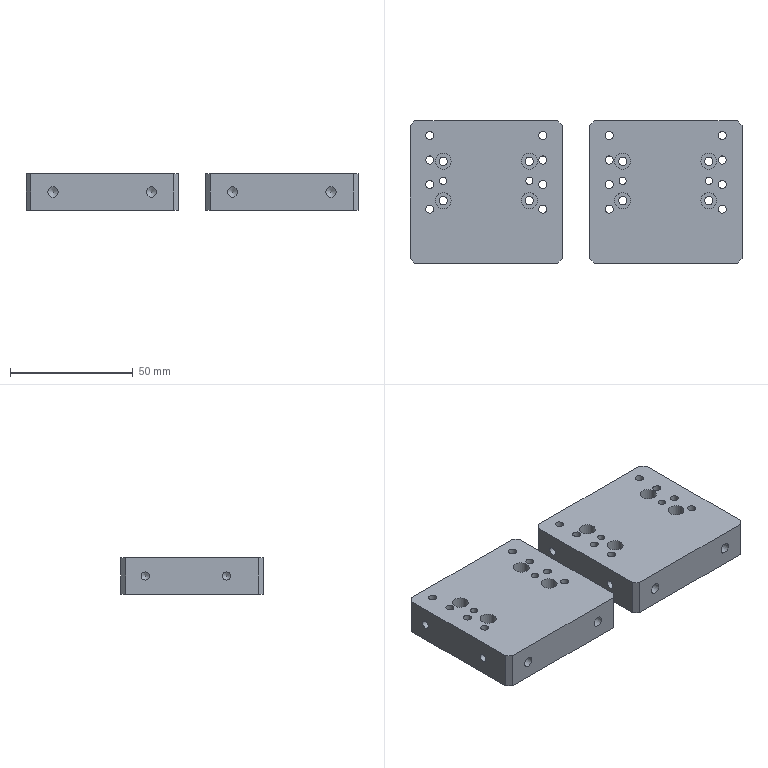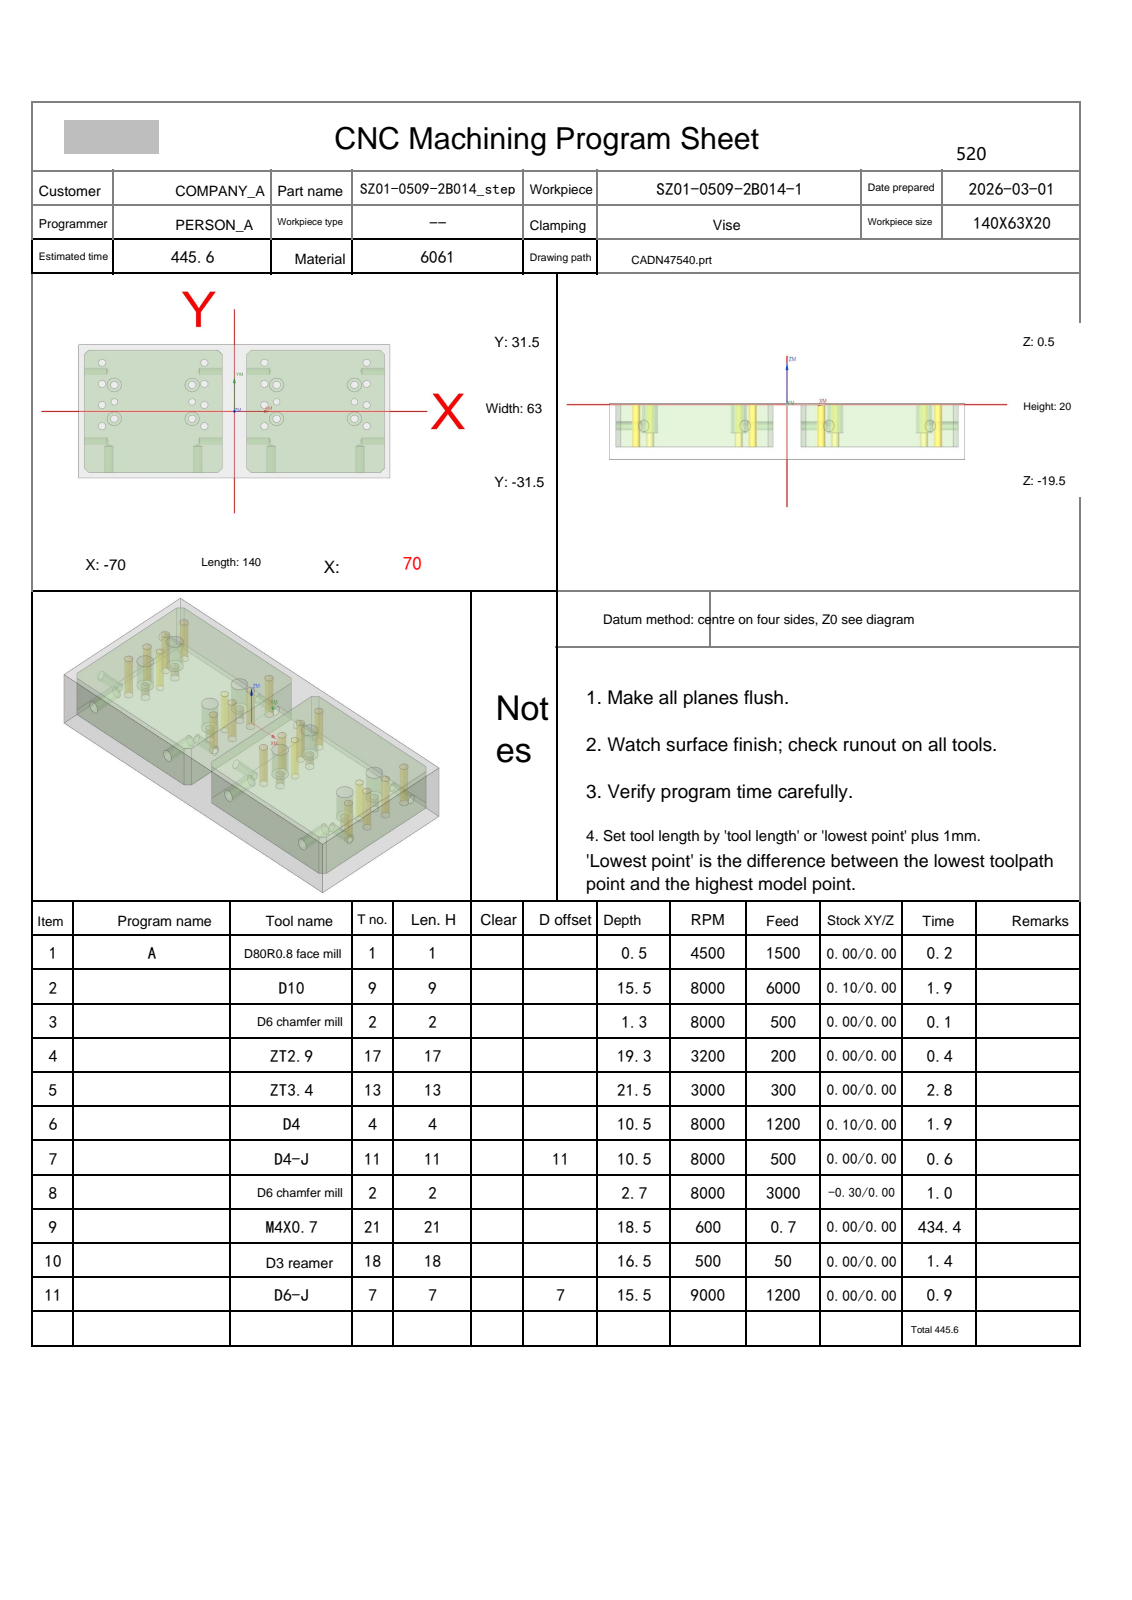NC program | NX | posted by the shop | part box 135 x 58 x 15 mm
Lines 1 to 1865 of 1983, first 1190 of 1863 lines:
%
O0001
(Machine time: 858.92 MIN)
(===Total Tool:10===)
(T1=D80R0.8 face mill D=80.  R=0.8  D-  H01 Z=0.    )
(T9=D10     D=10.  R=0.   D-  H09 Z=-15.  )
(T2=D6 chamfer mill   D=6.   R=0.   D-  H02 Z=-2.2  )
(T17=ZT2.9  D=2.9  DR_a=120 D-  H17 Z=-18.84)
(T13=ZT3.4  D=3.4  DR_a=118 D-  H13 Z=-21.  )
(T4=D4      D=4.   R=0.   D-  H04 Z=-10.  )
(T11=D4-J   D=4.   R=0.   D11 H11 Z=-10.  )
(T21=M4X0.7 D=3.3  DR_a=180 D-  H21 Z=-18.  )
(T18=D3 reamer   D=3.   DR_a=180 D-  H18 Z=-16.  )
(T7=D6-J    D=6.   R=0.   D7  H07 Z=-15.  )
G80 G90 G17 G49 G40
G91 G28 Z0
M01
N1 T01 M06
(D80R0.8 face mill  D=80. R=0.8 H=01 ce=0.00 di=0.00)
G00 G90 G54 X-112.5 Y0.0 M03 S4500
G43 H01 Z50.
M08
Z2.
G01 Z0.0 F1500.
X-107.5
X107.5
X112.5
Z2.
G00 Z50.
G91 G28 Z0.0
M05
M09
G91 G28 Z0.0
M01
N2 T09 M06
(D10  D=10. R=0. H=09 ce=0.10 di=0.00)
G00 G90 G54 X36.5 Y34.1 M03 S8000
G43 H09 Z50.
M08
Z.5
G01 X65.5 Z.416 F6000.
G02 X69.106 Y32.606 Z.404 I0.0 J-5.1
G01 X71.106 Y30.606 Z.396
G02 X72.6 Y27. Z.385 I-3.606 J-3.606
G01 Y-27. Z.228
G02 X71.106 Y-30.606 Z.216 I-5.1 J0.0
G01 X69.106 Y-32.606 Z.208
G02 X65.5 Y-34.1 Z.197 I-3.606 J3.606
G01 X7.5 Z.028
G02 X3.894 Y-32.606 Z.017 I0.0 J5.1
G01 X1.894 Y-30.606 Z.009
G02 X.4 Y-27. Z-.003 I3.606 J3.606
G01 Y27. Z-.16
G02 X1.894 Y30.606 Z-.171 I5.1 J0.0
G01 X3.894 Y32.606 Z-.179
G02 X7.5 Y34.1 Z-.191 I3.606 J-3.606
G01 X65.5 Z-.359
G02 X69.106 Y32.606 Z-.371 I0.0 J-5.1
G01 X71.106 Y30.606 Z-.379
G02 X72.6 Y27. Z-.39 I-3.606 J-3.606
G01 Y-27. Z-.547
G02 X71.106 Y-30.606 Z-.559 I-5.1 J0.0
G01 X69.106 Y-32.606 Z-.567
G02 X65.5 Y-34.1 Z-.578 I-3.606 J3.606
G01 X7.5 Z-.747
G02 X3.894 Y-32.606 Z-.758 I0.0 J5.1
G01 X1.894 Y-30.606 Z-.766
G02 X.4 Y-27. Z-.778 I3.606 J3.606
G01 Y27. Z-.935
G02 X1.894 Y30.606 Z-.946 I5.1 J0.0
G01 X3.894 Y32.606 Z-.954
G02 X7.5 Y34.1 Z-.966 I3.606 J-3.606
G01 X65.5 Z-1.134
G02 X69.106 Y32.606 Z-1.146 I0.0 J-5.1
G01 X71.106 Y30.606 Z-1.154
G02 X72.6 Y27. Z-1.165 I-3.606 J-3.606
G01 Y-27. Z-1.322
G02 X71.106 Y-30.606 Z-1.334 I-5.1 J0.0
G01 X69.106 Y-32.606 Z-1.342
G02 X65.5 Y-34.1 Z-1.353 I-3.606 J3.606
G01 X7.5 Z-1.522
G02 X3.894 Y-32.606 Z-1.533 I0.0 J5.1
G01 X1.894 Y-30.606 Z-1.541
G02 X.4 Y-27. Z-1.553 I3.606 J3.606
G01 Y27. Z-1.71
G02 X1.894 Y30.606 Z-1.721 I5.1 J0.0
G01 X3.894 Y32.606 Z-1.729
G02 X7.5 Y34.1 Z-1.741 I3.606 J-3.606
G01 X65.5 Z-1.909
G02 X69.106 Y32.606 Z-1.921 I0.0 J-5.1
G01 X71.106 Y30.606 Z-1.929
G02 X72.6 Y27. Z-1.94 I-3.606 J-3.606
G01 Y-27. Z-2.097
G02 X71.106 Y-30.606 Z-2.109 I-5.1 J0.0
G01 X69.106 Y-32.606 Z-2.117
G02 X65.5 Y-34.1 Z-2.128 I-3.606 J3.606
G01 X7.5 Z-2.297
G02 X3.894 Y-32.606 Z-2.308 I0.0 J5.1
G01 X1.894 Y-30.606 Z-2.316
G02 X.4 Y-27. Z-2.328 I3.606 J3.606
G01 Y27. Z-2.485
G02 X1.894 Y30.606 Z-2.496 I5.1 J0.0
G01 X3.894 Y32.606 Z-2.504
G02 X7.5 Y34.1 Z-2.516 I3.606 J-3.606
G01 X65.5 Z-2.684
G02 X69.106 Y32.606 Z-2.696 I0.0 J-5.1
G01 X71.106 Y30.606 Z-2.704
G02 X72.6 Y27. Z-2.715 I-3.606 J-3.606
G01 Y-27. Z-2.872
G02 X71.106 Y-30.606 Z-2.884 I-5.1 J0.0
G01 X69.106 Y-32.606 Z-2.892
G02 X65.5 Y-34.1 Z-2.903 I-3.606 J3.606
G01 X7.5 Z-3.072
G02 X3.894 Y-32.606 Z-3.083 I0.0 J5.1
G01 X1.894 Y-30.606 Z-3.091
G02 X.4 Y-27. Z-3.103 I3.606 J3.606
G01 Y27. Z-3.26
G02 X1.894 Y30.606 Z-3.271 I5.1 J0.0
G01 X3.894 Y32.606 Z-3.279
G02 X7.5 Y34.1 Z-3.291 I3.606 J-3.606
G01 X65.5 Z-3.459
G02 X69.106 Y32.606 Z-3.471 I0.0 J-5.1
G01 X71.106 Y30.606 Z-3.479
G02 X72.6 Y27. Z-3.49 I-3.606 J-3.606
G01 Y-27. Z-3.647
G02 X71.106 Y-30.606 Z-3.659 I-5.1 J0.0
G01 X69.106 Y-32.606 Z-3.667
G02 X65.5 Y-34.1 Z-3.678 I-3.606 J3.606
G01 X7.5 Z-3.847
G02 X3.894 Y-32.606 Z-3.858 I0.0 J5.1
G01 X1.894 Y-30.606 Z-3.866
G02 X.4 Y-27. Z-3.878 I3.606 J3.606
G01 Y27. Z-4.035
G02 X1.894 Y30.606 Z-4.046 I5.1 J0.0
G01 X3.894 Y32.606 Z-4.054
G02 X7.5 Y34.1 Z-4.066 I3.606 J-3.606
G01 X65.5 Z-4.234
G02 X69.106 Y32.606 Z-4.246 I0.0 J-5.1
G01 X71.106 Y30.606 Z-4.254
G02 X72.6 Y27. Z-4.265 I-3.606 J-3.606
G01 Y-27. Z-4.422
G02 X71.106 Y-30.606 Z-4.434 I-5.1 J0.0
G01 X69.106 Y-32.606 Z-4.442
G02 X65.5 Y-34.1 Z-4.453 I-3.606 J3.606
G01 X7.5 Z-4.622
G02 X3.894 Y-32.606 Z-4.633 I0.0 J5.1
G01 X1.894 Y-30.606 Z-4.641
G02 X.4 Y-27. Z-4.653 I3.606 J3.606
G01 Y27. Z-4.81
G02 X1.894 Y30.606 Z-4.821 I5.1 J0.0
G01 X3.894 Y32.606 Z-4.829
G02 X7.5 Y34.1 Z-4.841 I3.606 J-3.606
G01 X65.5 Z-5.009
G02 X69.106 Y32.606 Z-5.021 I0.0 J-5.1
G01 X71.106 Y30.606 Z-5.029
G02 X72.6 Y27. Z-5.04 I-3.606 J-3.606
G01 Y-27. Z-5.197
G02 X71.106 Y-30.606 Z-5.209 I-5.1 J0.0
G01 X69.106 Y-32.606 Z-5.217
G02 X65.5 Y-34.1 Z-5.228 I-3.606 J3.606
G01 X7.5 Z-5.397
G02 X3.894 Y-32.606 Z-5.408 I0.0 J5.1
G01 X1.894 Y-30.606 Z-5.416
G02 X.4 Y-27. Z-5.428 I3.606 J3.606
G01 Y27. Z-5.585
G02 X1.894 Y30.606 Z-5.596 I5.1 J0.0
G01 X3.894 Y32.606 Z-5.604
G02 X7.5 Y34.1 Z-5.616 I3.606 J-3.606
G01 X65.5 Z-5.784
G02 X69.106 Y32.606 Z-5.796 I0.0 J-5.1
G01 X71.106 Y30.606 Z-5.804
G02 X72.6 Y27. Z-5.815 I-3.606 J-3.606
G01 Y-27. Z-5.972
G02 X71.106 Y-30.606 Z-5.984 I-5.1 J0.0
G01 X69.106 Y-32.606 Z-5.992
G02 X65.5 Y-34.1 Z-6.003 I-3.606 J3.606
G01 X7.5 Z-6.172
G02 X3.894 Y-32.606 Z-6.183 I0.0 J5.1
G01 X1.894 Y-30.606 Z-6.191
G02 X.4 Y-27. Z-6.203 I3.606 J3.606
G01 Y27. Z-6.36
G02 X1.894 Y30.606 Z-6.371 I5.1 J0.0
G01 X3.894 Y32.606 Z-6.379
G02 X7.5 Y34.1 Z-6.391 I3.606 J-3.606
G01 X65.5 Z-6.559
G02 X69.106 Y32.606 Z-6.571 I0.0 J-5.1
G01 X71.106 Y30.606 Z-6.579
G02 X72.6 Y27. Z-6.59 I-3.606 J-3.606
G01 Y-27. Z-6.747
G02 X71.106 Y-30.606 Z-6.759 I-5.1 J0.0
G01 X69.106 Y-32.606 Z-6.767
G02 X65.5 Y-34.1 Z-6.778 I-3.606 J3.606
G01 X7.5 Z-6.947
G02 X3.894 Y-32.606 Z-6.958 I0.0 J5.1
G01 X1.894 Y-30.606 Z-6.966
G02 X.4 Y-27. Z-6.978 I3.606 J3.606
G01 Y27. Z-7.135
G02 X1.894 Y30.606 Z-7.146 I5.1 J0.0
G01 X3.894 Y32.606 Z-7.154
G02 X7.5 Y34.1 Z-7.166 I3.606 J-3.606
G01 X65.5 Z-7.334
G02 X69.106 Y32.606 Z-7.346 I0.0 J-5.1
G01 X71.106 Y30.606 Z-7.354
G02 X72.6 Y27. Z-7.365 I-3.606 J-3.606
G01 Y-27. Z-7.522
G02 X71.106 Y-30.606 Z-7.534 I-5.1 J0.0
G01 X69.106 Y-32.606 Z-7.542
G02 X65.5 Y-34.1 Z-7.553 I-3.606 J3.606
G01 X7.5 Z-7.722
G02 X3.894 Y-32.606 Z-7.733 I0.0 J5.1
G01 X1.894 Y-30.606 Z-7.741
G02 X.4 Y-27. Z-7.753 I3.606 J3.606
G01 Y27. Z-7.91
G02 X1.894 Y30.606 Z-7.921 I5.1 J0.0
G01 X3.894 Y32.606 Z-7.929
G02 X7.5 Y34.1 Z-7.941 I3.606 J-3.606
G01 X65.5 Z-8.109
G02 X69.106 Y32.606 Z-8.121 I0.0 J-5.1
G01 X71.106 Y30.606 Z-8.129
G02 X72.6 Y27. Z-8.14 I-3.606 J-3.606
G01 Y-27. Z-8.297
G02 X71.106 Y-30.606 Z-8.309 I-5.1 J0.0
G01 X69.106 Y-32.606 Z-8.317
G02 X65.5 Y-34.1 Z-8.328 I-3.606 J3.606
G01 X7.5 Z-8.497
G02 X3.894 Y-32.606 Z-8.508 I0.0 J5.1
G01 X1.894 Y-30.606 Z-8.516
G02 X.4 Y-27. Z-8.528 I3.606 J3.606
G01 Y27. Z-8.685
G02 X1.894 Y30.606 Z-8.696 I5.1 J0.0
G01 X3.894 Y32.606 Z-8.704
G02 X7.5 Y34.1 Z-8.716 I3.606 J-3.606
G01 X65.5 Z-8.884
G02 X69.106 Y32.606 Z-8.896 I0.0 J-5.1
G01 X71.106 Y30.606 Z-8.904
G02 X72.6 Y27. Z-8.915 I-3.606 J-3.606
G01 Y-27. Z-9.072
G02 X71.106 Y-30.606 Z-9.084 I-5.1 J0.0
G01 X69.106 Y-32.606 Z-9.092
G02 X65.5 Y-34.1 Z-9.103 I-3.606 J3.606
G01 X7.5 Z-9.272
G02 X3.894 Y-32.606 Z-9.283 I0.0 J5.1
G01 X1.894 Y-30.606 Z-9.291
G02 X.4 Y-27. Z-9.303 I3.606 J3.606
G01 Y27. Z-9.46
G02 X1.894 Y30.606 Z-9.471 I5.1 J0.0
G01 X3.894 Y32.606 Z-9.479
G02 X7.5 Y34.1 Z-9.491 I3.606 J-3.606
G01 X65.5 Z-9.659
G02 X69.106 Y32.606 Z-9.671 I0.0 J-5.1
G01 X71.106 Y30.606 Z-9.679
G02 X72.6 Y27. Z-9.69 I-3.606 J-3.606
G01 Y-27. Z-9.847
G02 X71.106 Y-30.606 Z-9.859 I-5.1 J0.0
G01 X69.106 Y-32.606 Z-9.867
G02 X65.5 Y-34.1 Z-9.878 I-3.606 J3.606
G01 X7.5 Z-10.047
G02 X3.894 Y-32.606 Z-10.058 I0.0 J5.1
G01 X1.894 Y-30.606 Z-10.066
G02 X.4 Y-27. Z-10.078 I3.606 J3.606
G01 Y27. Z-10.235
G02 X1.894 Y30.606 Z-10.246 I5.1 J0.0
G01 X3.894 Y32.606 Z-10.254
G02 X7.5 Y34.1 Z-10.266 I3.606 J-3.606
G01 X65.5 Z-10.434
G02 X69.106 Y32.606 Z-10.446 I0.0 J-5.1
G01 X71.106 Y30.606 Z-10.454
G02 X72.6 Y27. Z-10.465 I-3.606 J-3.606
G01 Y-27. Z-10.622
G02 X71.106 Y-30.606 Z-10.634 I-5.1 J0.0
G01 X69.106 Y-32.606 Z-10.642
G02 X65.5 Y-34.1 Z-10.653 I-3.606 J3.606
G01 X7.5 Z-10.822
G02 X3.894 Y-32.606 Z-10.833 I0.0 J5.1
G01 X1.894 Y-30.606 Z-10.841
G02 X.4 Y-27. Z-10.853 I3.606 J3.606
G01 Y27. Z-11.01
G02 X1.894 Y30.606 Z-11.021 I5.1 J0.0
G01 X3.894 Y32.606 Z-11.029
G02 X7.5 Y34.1 Z-11.041 I3.606 J-3.606
G01 X65.5 Z-11.209
G02 X69.106 Y32.606 Z-11.221 I0.0 J-5.1
G01 X71.106 Y30.606 Z-11.229
G02 X72.6 Y27. Z-11.24 I-3.606 J-3.606
G01 Y-27. Z-11.397
G02 X71.106 Y-30.606 Z-11.409 I-5.1 J0.0
G01 X69.106 Y-32.606 Z-11.417
G02 X65.5 Y-34.1 Z-11.428 I-3.606 J3.606
G01 X7.5 Z-11.597
G02 X3.894 Y-32.606 Z-11.608 I0.0 J5.1
G01 X1.894 Y-30.606 Z-11.616
G02 X.4 Y-27. Z-11.628 I3.606 J3.606
G01 Y27. Z-11.785
G02 X1.894 Y30.606 Z-11.796 I5.1 J0.0
G01 X3.894 Y32.606 Z-11.804
G02 X7.5 Y34.1 Z-11.816 I3.606 J-3.606
G01 X65.5 Z-11.984
G02 X69.106 Y32.606 Z-11.996 I0.0 J-5.1
G01 X71.106 Y30.606 Z-12.004
G02 X72.6 Y27. Z-12.015 I-3.606 J-3.606
G01 Y-27. Z-12.172
G02 X71.106 Y-30.606 Z-12.184 I-5.1 J0.0
G01 X69.106 Y-32.606 Z-12.192
G02 X65.5 Y-34.1 Z-12.203 I-3.606 J3.606
G01 X7.5 Z-12.372
G02 X3.894 Y-32.606 Z-12.383 I0.0 J5.1
G01 X1.894 Y-30.606 Z-12.391
G02 X.4 Y-27. Z-12.403 I3.606 J3.606
G01 Y27. Z-12.56
G02 X1.894 Y30.606 Z-12.571 I5.1 J0.0
G01 X3.894 Y32.606 Z-12.579
G02 X7.5 Y34.1 Z-12.591 I3.606 J-3.606
G01 X65.5 Z-12.759
G02 X69.106 Y32.606 Z-12.771 I0.0 J-5.1
G01 X71.106 Y30.606 Z-12.779
G02 X72.6 Y27. Z-12.79 I-3.606 J-3.606
G01 Y-27. Z-12.947
G02 X71.106 Y-30.606 Z-12.959 I-5.1 J0.0
G01 X69.106 Y-32.606 Z-12.967
G02 X65.5 Y-34.1 Z-12.978 I-3.606 J3.606
G01 X7.5 Z-13.147
G02 X3.894 Y-32.606 Z-13.158 I0.0 J5.1
G01 X1.894 Y-30.606 Z-13.166
G02 X.4 Y-27. Z-13.178 I3.606 J3.606
G01 Y27. Z-13.335
G02 X1.894 Y30.606 Z-13.346 I5.1 J0.0
G01 X3.894 Y32.606 Z-13.354
G02 X7.5 Y34.1 Z-13.366 I3.606 J-3.606
G01 X65.5 Z-13.534
G02 X69.106 Y32.606 Z-13.546 I0.0 J-5.1
G01 X71.106 Y30.606 Z-13.554
G02 X72.6 Y27. Z-13.565 I-3.606 J-3.606
G01 Y-27. Z-13.722
G02 X71.106 Y-30.606 Z-13.734 I-5.1 J0.0
G01 X69.106 Y-32.606 Z-13.742
G02 X65.5 Y-34.1 Z-13.753 I-3.606 J3.606
G01 X7.5 Z-13.922
G02 X3.894 Y-32.606 Z-13.933 I0.0 J5.1
G01 X1.894 Y-30.606 Z-13.941
G02 X.4 Y-27. Z-13.953 I3.606 J3.606
G01 Y27. Z-14.11
G02 X1.894 Y30.606 Z-14.121 I5.1 J0.0
G01 X3.894 Y32.606 Z-14.129
G02 X7.5 Y34.1 Z-14.141 I3.606 J-3.606
G01 X65.5 Z-14.309
G02 X69.106 Y32.606 Z-14.321 I0.0 J-5.1
G01 X71.106 Y30.606 Z-14.329
G02 X72.6 Y27. Z-14.34 I-3.606 J-3.606
G01 Y-27. Z-14.497
G02 X71.106 Y-30.606 Z-14.509 I-5.1 J0.0
G01 X69.106 Y-32.606 Z-14.517
G02 X65.5 Y-34.1 Z-14.528 I-3.606 J3.606
G01 X7.5 Z-14.697
G02 X3.894 Y-32.606 Z-14.708 I0.0 J5.1
G01 X1.894 Y-30.606 Z-14.716
G02 X.4 Y-27. Z-14.728 I3.606 J3.606
G01 Y27. Z-14.885
G02 X1.894 Y30.606 Z-14.896 I5.1 J0.0
G01 X3.894 Y32.606 Z-14.904
G02 X7.5 Y34.1 Z-14.916 I3.606 J-3.606
G01 X36.5 Z-15.
X65.5
G02 X69.106 Y32.606 I0.0 J-5.1
G01 X71.106 Y30.606
G02 X72.6 Y27. I-3.606 J-3.606
G01 Y-27.
G02 X71.106 Y-30.606 I-5.1 J0.0
G01 X69.106 Y-32.606
G02 X65.5 Y-34.1 I-3.606 J3.606
G01 X7.5
G02 X3.894 Y-32.606 I0.0 J5.1
G01 X1.894 Y-30.606
G02 X.4 Y-27. I3.606 J3.606
G01 Y27.
G02 X1.894 Y30.606 I5.1 J0.0
G01 X3.894 Y32.606
G02 X7.5 Y34.1 I3.606 J-3.606
G01 X36.5
X37.
Z-14.
G00 Z50.
X-36.5
Z.5
G01 X-7.5 Z.416
G02 X-3.894 Y32.606 Z.404 I0.0 J-5.1
G01 X-1.894 Y30.606 Z.396
G02 X-.4 Y27. Z.385 I-3.606 J-3.606
G01 Y-27. Z.228
G02 X-1.894 Y-30.606 Z.216 I-5.1 J0.0
G01 X-3.894 Y-32.606 Z.208
G02 X-7.5 Y-34.1 Z.197 I-3.606 J3.606
G01 X-65.5 Z.028
G02 X-69.106 Y-32.606 Z.017 I0.0 J5.1
G01 X-71.106 Y-30.606 Z.009
G02 X-72.6 Y-27. Z-.003 I3.606 J3.606
G01 Y27. Z-.16
G02 X-71.106 Y30.606 Z-.171 I5.1 J0.0
G01 X-69.106 Y32.606 Z-.179
G02 X-65.5 Y34.1 Z-.191 I3.606 J-3.606
G01 X-7.5 Z-.359
G02 X-3.894 Y32.606 Z-.371 I0.0 J-5.1
G01 X-1.894 Y30.606 Z-.379
G02 X-.4 Y27. Z-.39 I-3.606 J-3.606
G01 Y-27. Z-.547
G02 X-1.894 Y-30.606 Z-.559 I-5.1 J0.0
G01 X-3.894 Y-32.606 Z-.567
G02 X-7.5 Y-34.1 Z-.578 I-3.606 J3.606
G01 X-65.5 Z-.747
G02 X-69.106 Y-32.606 Z-.758 I0.0 J5.1
G01 X-71.106 Y-30.606 Z-.766
G02 X-72.6 Y-27. Z-.778 I3.606 J3.606
G01 Y27. Z-.935
G02 X-71.106 Y30.606 Z-.946 I5.1 J0.0
G01 X-69.106 Y32.606 Z-.954
G02 X-65.5 Y34.1 Z-.966 I3.606 J-3.606
G01 X-7.5 Z-1.134
G02 X-3.894 Y32.606 Z-1.146 I0.0 J-5.1
G01 X-1.894 Y30.606 Z-1.154
G02 X-.4 Y27. Z-1.165 I-3.606 J-3.606
G01 Y-27. Z-1.322
G02 X-1.894 Y-30.606 Z-1.334 I-5.1 J0.0
G01 X-3.894 Y-32.606 Z-1.342
G02 X-7.5 Y-34.1 Z-1.353 I-3.606 J3.606
G01 X-65.5 Z-1.522
G02 X-69.106 Y-32.606 Z-1.533 I0.0 J5.1
G01 X-71.106 Y-30.606 Z-1.541
G02 X-72.6 Y-27. Z-1.553 I3.606 J3.606
G01 Y27. Z-1.71
G02 X-71.106 Y30.606 Z-1.721 I5.1 J0.0
G01 X-69.106 Y32.606 Z-1.729
G02 X-65.5 Y34.1 Z-1.741 I3.606 J-3.606
G01 X-7.5 Z-1.909
G02 X-3.894 Y32.606 Z-1.921 I0.0 J-5.1
G01 X-1.894 Y30.606 Z-1.929
G02 X-.4 Y27. Z-1.94 I-3.606 J-3.606
G01 Y-27. Z-2.097
G02 X-1.894 Y-30.606 Z-2.109 I-5.1 J0.0
G01 X-3.894 Y-32.606 Z-2.117
G02 X-7.5 Y-34.1 Z-2.128 I-3.606 J3.606
G01 X-65.5 Z-2.297
G02 X-69.106 Y-32.606 Z-2.308 I0.0 J5.1
G01 X-71.106 Y-30.606 Z-2.316
G02 X-72.6 Y-27. Z-2.328 I3.606 J3.606
G01 Y27. Z-2.485
G02 X-71.106 Y30.606 Z-2.496 I5.1 J0.0
G01 X-69.106 Y32.606 Z-2.504
G02 X-65.5 Y34.1 Z-2.516 I3.606 J-3.606
G01 X-7.5 Z-2.684
G02 X-3.894 Y32.606 Z-2.696 I0.0 J-5.1
G01 X-1.894 Y30.606 Z-2.704
G02 X-.4 Y27. Z-2.715 I-3.606 J-3.606
G01 Y-27. Z-2.872
G02 X-1.894 Y-30.606 Z-2.884 I-5.1 J0.0
G01 X-3.894 Y-32.606 Z-2.892
G02 X-7.5 Y-34.1 Z-2.903 I-3.606 J3.606
G01 X-65.5 Z-3.072
G02 X-69.106 Y-32.606 Z-3.083 I0.0 J5.1
G01 X-71.106 Y-30.606 Z-3.091
G02 X-72.6 Y-27. Z-3.103 I3.606 J3.606
G01 Y27. Z-3.26
G02 X-71.106 Y30.606 Z-3.271 I5.1 J0.0
G01 X-69.106 Y32.606 Z-3.279
G02 X-65.5 Y34.1 Z-3.291 I3.606 J-3.606
G01 X-7.5 Z-3.459
G02 X-3.894 Y32.606 Z-3.471 I0.0 J-5.1
G01 X-1.894 Y30.606 Z-3.479
G02 X-.4 Y27. Z-3.49 I-3.606 J-3.606
G01 Y-27. Z-3.647
G02 X-1.894 Y-30.606 Z-3.659 I-5.1 J0.0
G01 X-3.894 Y-32.606 Z-3.667
G02 X-7.5 Y-34.1 Z-3.678 I-3.606 J3.606
G01 X-65.5 Z-3.847
G02 X-69.106 Y-32.606 Z-3.858 I0.0 J5.1
G01 X-71.106 Y-30.606 Z-3.866
G02 X-72.6 Y-27. Z-3.878 I3.606 J3.606
G01 Y27. Z-4.035
G02 X-71.106 Y30.606 Z-4.046 I5.1 J0.0
G01 X-69.106 Y32.606 Z-4.054
G02 X-65.5 Y34.1 Z-4.066 I3.606 J-3.606
G01 X-7.5 Z-4.234
G02 X-3.894 Y32.606 Z-4.246 I0.0 J-5.1
G01 X-1.894 Y30.606 Z-4.254
G02 X-.4 Y27. Z-4.265 I-3.606 J-3.606
G01 Y-27. Z-4.422
G02 X-1.894 Y-30.606 Z-4.434 I-5.1 J0.0
G01 X-3.894 Y-32.606 Z-4.442
G02 X-7.5 Y-34.1 Z-4.453 I-3.606 J3.606
G01 X-65.5 Z-4.622
G02 X-69.106 Y-32.606 Z-4.633 I0.0 J5.1
G01 X-71.106 Y-30.606 Z-4.641
G02 X-72.6 Y-27. Z-4.653 I3.606 J3.606
G01 Y27. Z-4.81
G02 X-71.106 Y30.606 Z-4.821 I5.1 J0.0
G01 X-69.106 Y32.606 Z-4.829
G02 X-65.5 Y34.1 Z-4.841 I3.606 J-3.606
G01 X-7.5 Z-5.009
G02 X-3.894 Y32.606 Z-5.021 I0.0 J-5.1
G01 X-1.894 Y30.606 Z-5.029
G02 X-.4 Y27. Z-5.04 I-3.606 J-3.606
G01 Y-27. Z-5.197
G02 X-1.894 Y-30.606 Z-5.209 I-5.1 J0.0
G01 X-3.894 Y-32.606 Z-5.217
G02 X-7.5 Y-34.1 Z-5.228 I-3.606 J3.606
G01 X-65.5 Z-5.397
G02 X-69.106 Y-32.606 Z-5.408 I0.0 J5.1
G01 X-71.106 Y-30.606 Z-5.416
G02 X-72.6 Y-27. Z-5.428 I3.606 J3.606
G01 Y27. Z-5.585
G02 X-71.106 Y30.606 Z-5.596 I5.1 J0.0
G01 X-69.106 Y32.606 Z-5.604
G02 X-65.5 Y34.1 Z-5.616 I3.606 J-3.606
G01 X-7.5 Z-5.784
G02 X-3.894 Y32.606 Z-5.796 I0.0 J-5.1
G01 X-1.894 Y30.606 Z-5.804
G02 X-.4 Y27. Z-5.815 I-3.606 J-3.606
G01 Y-27. Z-5.972
G02 X-1.894 Y-30.606 Z-5.984 I-5.1 J0.0
G01 X-3.894 Y-32.606 Z-5.992
G02 X-7.5 Y-34.1 Z-6.003 I-3.606 J3.606
G01 X-65.5 Z-6.172
G02 X-69.106 Y-32.606 Z-6.183 I0.0 J5.1
G01 X-71.106 Y-30.606 Z-6.191
G02 X-72.6 Y-27. Z-6.203 I3.606 J3.606
G01 Y27. Z-6.36
G02 X-71.106 Y30.606 Z-6.371 I5.1 J0.0
G01 X-69.106 Y32.606 Z-6.379
G02 X-65.5 Y34.1 Z-6.391 I3.606 J-3.606
G01 X-7.5 Z-6.559
G02 X-3.894 Y32.606 Z-6.571 I0.0 J-5.1
G01 X-1.894 Y30.606 Z-6.579
G02 X-.4 Y27. Z-6.59 I-3.606 J-3.606
G01 Y-27. Z-6.747
G02 X-1.894 Y-30.606 Z-6.759 I-5.1 J0.0
G01 X-3.894 Y-32.606 Z-6.767
G02 X-7.5 Y-34.1 Z-6.778 I-3.606 J3.606
G01 X-65.5 Z-6.947
G02 X-69.106 Y-32.606 Z-6.958 I0.0 J5.1
G01 X-71.106 Y-30.606 Z-6.966
G02 X-72.6 Y-27. Z-6.978 I3.606 J3.606
G01 Y27. Z-7.135
G02 X-71.106 Y30.606 Z-7.146 I5.1 J0.0
G01 X-69.106 Y32.606 Z-7.154
G02 X-65.5 Y34.1 Z-7.166 I3.606 J-3.606
G01 X-7.5 Z-7.334
G02 X-3.894 Y32.606 Z-7.346 I0.0 J-5.1
G01 X-1.894 Y30.606 Z-7.354
G02 X-.4 Y27. Z-7.365 I-3.606 J-3.606
G01 Y-27. Z-7.522
G02 X-1.894 Y-30.606 Z-7.534 I-5.1 J0.0
G01 X-3.894 Y-32.606 Z-7.542
G02 X-7.5 Y-34.1 Z-7.553 I-3.606 J3.606
G01 X-65.5 Z-7.722
G02 X-69.106 Y-32.606 Z-7.733 I0.0 J5.1
G01 X-71.106 Y-30.606 Z-7.741
G02 X-72.6 Y-27. Z-7.753 I3.606 J3.606
G01 Y27. Z-7.91
G02 X-71.106 Y30.606 Z-7.921 I5.1 J0.0
G01 X-69.106 Y32.606 Z-7.929
G02 X-65.5 Y34.1 Z-7.941 I3.606 J-3.606
G01 X-7.5 Z-8.109
G02 X-3.894 Y32.606 Z-8.121 I0.0 J-5.1
G01 X-1.894 Y30.606 Z-8.129
G02 X-.4 Y27. Z-8.14 I-3.606 J-3.606
G01 Y-27. Z-8.297
G02 X-1.894 Y-30.606 Z-8.309 I-5.1 J0.0
G01 X-3.894 Y-32.606 Z-8.317
G02 X-7.5 Y-34.1 Z-8.328 I-3.606 J3.606
G01 X-65.5 Z-8.497
G02 X-69.106 Y-32.606 Z-8.508 I0.0 J5.1
G01 X-71.106 Y-30.606 Z-8.516
G02 X-72.6 Y-27. Z-8.528 I3.606 J3.606
G01 Y27. Z-8.685
G02 X-71.106 Y30.606 Z-8.696 I5.1 J0.0
G01 X-69.106 Y32.606 Z-8.704
G02 X-65.5 Y34.1 Z-8.716 I3.606 J-3.606
G01 X-7.5 Z-8.884
G02 X-3.894 Y32.606 Z-8.896 I0.0 J-5.1
G01 X-1.894 Y30.606 Z-8.904
G02 X-.4 Y27. Z-8.915 I-3.606 J-3.606
G01 Y-27. Z-9.072
G02 X-1.894 Y-30.606 Z-9.084 I-5.1 J0.0
G01 X-3.894 Y-32.606 Z-9.092
G02 X-7.5 Y-34.1 Z-9.103 I-3.606 J3.606
G01 X-65.5 Z-9.272
G02 X-69.106 Y-32.606 Z-9.283 I0.0 J5.1
G01 X-71.106 Y-30.606 Z-9.291
G02 X-72.6 Y-27. Z-9.303 I3.606 J3.606
G01 Y27. Z-9.46
G02 X-71.106 Y30.606 Z-9.471 I5.1 J0.0
G01 X-69.106 Y32.606 Z-9.479
G02 X-65.5 Y34.1 Z-9.491 I3.606 J-3.606
G01 X-7.5 Z-9.659
G02 X-3.894 Y32.606 Z-9.671 I0.0 J-5.1
G01 X-1.894 Y30.606 Z-9.679
G02 X-.4 Y27. Z-9.69 I-3.606 J-3.606
G01 Y-27. Z-9.847
G02 X-1.894 Y-30.606 Z-9.859 I-5.1 J0.0
G01 X-3.894 Y-32.606 Z-9.867
G02 X-7.5 Y-34.1 Z-9.878 I-3.606 J3.606
G01 X-65.5 Z-10.047
G02 X-69.106 Y-32.606 Z-10.058 I0.0 J5.1
G01 X-71.106 Y-30.606 Z-10.066
G02 X-72.6 Y-27. Z-10.078 I3.606 J3.606
G01 Y27. Z-10.235
G02 X-71.106 Y30.606 Z-10.246 I5.1 J0.0
G01 X-69.106 Y32.606 Z-10.254
G02 X-65.5 Y34.1 Z-10.266 I3.606 J-3.606
G01 X-7.5 Z-10.434
G02 X-3.894 Y32.606 Z-10.446 I0.0 J-5.1
G01 X-1.894 Y30.606 Z-10.454
G02 X-.4 Y27. Z-10.465 I-3.606 J-3.606
G01 Y-27. Z-10.622
G02 X-1.894 Y-30.606 Z-10.634 I-5.1 J0.0
G01 X-3.894 Y-32.606 Z-10.642
G02 X-7.5 Y-34.1 Z-10.653 I-3.606 J3.606
G01 X-65.5 Z-10.822
G02 X-69.106 Y-32.606 Z-10.833 I0.0 J5.1
G01 X-71.106 Y-30.606 Z-10.841
G02 X-72.6 Y-27. Z-10.853 I3.606 J3.606
G01 Y27. Z-11.01
G02 X-71.106 Y30.606 Z-11.021 I5.1 J0.0
G01 X-69.106 Y32.606 Z-11.029
G02 X-65.5 Y34.1 Z-11.041 I3.606 J-3.606
G01 X-7.5 Z-11.209
G02 X-3.894 Y32.606 Z-11.221 I0.0 J-5.1
G01 X-1.894 Y30.606 Z-11.229
G02 X-.4 Y27. Z-11.24 I-3.606 J-3.606
G01 Y-27. Z-11.397
G02 X-1.894 Y-30.606 Z-11.409 I-5.1 J0.0
G01 X-3.894 Y-32.606 Z-11.417
G02 X-7.5 Y-34.1 Z-11.428 I-3.606 J3.606
G01 X-65.5 Z-11.597
G02 X-69.106 Y-32.606 Z-11.608 I0.0 J5.1
G01 X-71.106 Y-30.606 Z-11.616
G02 X-72.6 Y-27. Z-11.628 I3.606 J3.606
G01 Y27. Z-11.785
G02 X-71.106 Y30.606 Z-11.796 I5.1 J0.0
G01 X-69.106 Y32.606 Z-11.804
G02 X-65.5 Y34.1 Z-11.816 I3.606 J-3.606
G01 X-7.5 Z-11.984
G02 X-3.894 Y32.606 Z-11.996 I0.0 J-5.1
G01 X-1.894 Y30.606 Z-12.004
G02 X-.4 Y27. Z-12.015 I-3.606 J-3.606
G01 Y-27. Z-12.172
G02 X-1.894 Y-30.606 Z-12.184 I-5.1 J0.0
G01 X-3.894 Y-32.606 Z-12.192
G02 X-7.5 Y-34.1 Z-12.203 I-3.606 J3.606
G01 X-65.5 Z-12.372
G02 X-69.106 Y-32.606 Z-12.383 I0.0 J5.1
G01 X-71.106 Y-30.606 Z-12.391
G02 X-72.6 Y-27. Z-12.403 I3.606 J3.606
G01 Y27. Z-12.56
G02 X-71.106 Y30.606 Z-12.571 I5.1 J0.0
G01 X-69.106 Y32.606 Z-12.579
G02 X-65.5 Y34.1 Z-12.591 I3.606 J-3.606
G01 X-7.5 Z-12.759
G02 X-3.894 Y32.606 Z-12.771 I0.0 J-5.1
G01 X-1.894 Y30.606 Z-12.779
G02 X-.4 Y27. Z-12.79 I-3.606 J-3.606
G01 Y-27. Z-12.947
G02 X-1.894 Y-30.606 Z-12.959 I-5.1 J0.0
G01 X-3.894 Y-32.606 Z-12.967
G02 X-7.5 Y-34.1 Z-12.978 I-3.606 J3.606
G01 X-65.5 Z-13.147
G02 X-69.106 Y-32.606 Z-13.158 I0.0 J5.1
G01 X-71.106 Y-30.606 Z-13.166
G02 X-72.6 Y-27. Z-13.178 I3.606 J3.606
G01 Y27. Z-13.335
G02 X-71.106 Y30.606 Z-13.346 I5.1 J0.0
G01 X-69.106 Y32.606 Z-13.354
G02 X-65.5 Y34.1 Z-13.366 I3.606 J-3.606
G01 X-7.5 Z-13.534
G02 X-3.894 Y32.606 Z-13.546 I0.0 J-5.1
G01 X-1.894 Y30.606 Z-13.554
G02 X-.4 Y27. Z-13.565 I-3.606 J-3.606
G01 Y-27. Z-13.722
G02 X-1.894 Y-30.606 Z-13.734 I-5.1 J0.0
G01 X-3.894 Y-32.606 Z-13.742
G02 X-7.5 Y-34.1 Z-13.753 I-3.606 J3.606
G01 X-65.5 Z-13.922
G02 X-69.106 Y-32.606 Z-13.933 I0.0 J5.1
G01 X-71.106 Y-30.606 Z-13.941
G02 X-72.6 Y-27. Z-13.953 I3.606 J3.606
G01 Y27. Z-14.11
G02 X-71.106 Y30.606 Z-14.121 I5.1 J0.0
G01 X-69.106 Y32.606 Z-14.129
G02 X-65.5 Y34.1 Z-14.141 I3.606 J-3.606
G01 X-7.5 Z-14.309
G02 X-3.894 Y32.606 Z-14.321 I0.0 J-5.1
G01 X-1.894 Y30.606 Z-14.329
G02 X-.4 Y27. Z-14.34 I-3.606 J-3.606
G01 Y-27. Z-14.497
G02 X-1.894 Y-30.606 Z-14.509 I-5.1 J0.0
G01 X-3.894 Y-32.606 Z-14.517
G02 X-7.5 Y-34.1 Z-14.528 I-3.606 J3.606
G01 X-65.5 Z-14.697
G02 X-69.106 Y-32.606 Z-14.708 I0.0 J5.1
G01 X-71.106 Y-30.606 Z-14.716
G02 X-72.6 Y-27. Z-14.728 I3.606 J3.606
G01 Y27. Z-14.885
G02 X-71.106 Y30.606 Z-14.896 I5.1 J0.0
G01 X-69.106 Y32.606 Z-14.904
G02 X-65.5 Y34.1 Z-14.916 I3.606 J-3.606
G01 X-36.5 Z-15.
X-7.5
G02 X-3.894 Y32.606 I0.0 J-5.1
G01 X-1.894 Y30.606
G02 X-.4 Y27. I-3.606 J-3.606
G01 Y-27.
G02 X-1.894 Y-30.606 I-5.1 J0.0
G01 X-3.894 Y-32.606
G02 X-7.5 Y-34.1 I-3.606 J3.606
G01 X-65.5
G02 X-69.106 Y-32.606 I0.0 J5.1
G01 X-71.106 Y-30.606
G02 X-72.6 Y-27. I3.606 J3.606
G01 Y27.
G02 X-71.106 Y30.606 I5.1 J0.0
G01 X-69.106 Y32.606
G02 X-65.5 Y34.1 I3.606 J-3.606
G01 X-36.5
X-36.
Z-14.
G00 Z50.
G91 G28 Z0.0
M05
M09
G91 G28 Z0.0
M01
N3 T02 M06
(D6 chamfer mill  D=6. R=0. H=02 ce=0.00 di=0.00)
G00 G90 G54 X-59.5 Y23. M03 S8000
G43 H02 Z50.
M08
G98 G81 X-59.5 Y23. Z-.8 R1. F500.
Y13.
X-54. Y12.5
Y4.5
X-59.5 Y3.
Y-7.
X-54. Y-3.5
X-19.
X-13.5 Y-7.
Y3.
X-19. Y4.5
Y12.5
X-13.5 Y13.
Y23.
X13.5
Y13.
X19. Y12.5
Y4.5
X13.5 Y3.
Y-7.
X19. Y-3.5
X54.
X59.5 Y-7.
Y3.
X54. Y4.5
Y12.5
X59.5 Y13.
Y23.
G80
G00 Z50.
G91 G28 Z0.0
M05
M09
G91 G28 Z0.0
M01
N4 T17 M06
(ZT2.9 D=2.9 DR_a=120 H=17)
G00 G90 G54 X54. Y4.5 M03 S3200
G43 H17 Z50.
M08
G98 G83 X54. Y4.5 Z-18.837 R1. F200. Q2.
X19.
X-19.
X-54.
G80
G00 Z50.
G91 G28 Z0.0
M05
M09
G91 G28 Z0.0
M01
N5 T13 M06
(ZT3.4 D=3.4 DR_a=118 H=13)
G00 G90 G54 X59.5 Y23. M03 S3000
G43 H13 Z50.
M08
G98 G83 X59.5 Y23. Z-21. R1. F300. Q2.
Y13.
Y3.
Y-7.
X13.5
Y3.
Y13.
Y23.
X-13.5
Y13.
Y3.
Y-7.
X-59.5
Y3.
Y13.
Y23.
G80
G00 Z50.
G00 G90 X54. Y12.5 M03 S2800
Z50.
G98 G83 X54. Y12.5 Z-18.021 R1. F100. Q2.
Y-3.5
X19.
Y12.5
X-19.
Y-3.5
X-54.
Y12.5
G80
G00 Z50.
G91 G28 Z0.0
M05
M09
G91 G28 Z0.0
M01
N6 T04 M06
(D4  D=4. R=0. H=04 ce=0.10 di=0.00)
G00 G90 G54 X19. Y12.5 M03 S8000
G43 H04 Z50.
M08
Z.5
G03 X19.575 Y11.925 I.575 J0.0 F1200.
X20.15 Y12.5 I0.0 J.575
X20.15 Y12.5 Z.2 I-1.15 J0.0
X20.15 Y12.5 Z-.1 I-1.15 J0.0
X20.15 Y12.5 Z-.4 I-1.15 J0.0
X20.15 Y12.5 Z-.7 I-1.15 J0.0
X20.15 Y12.5 Z-1. I-1.15 J0.0
X20.15 Y12.5 Z-1.3 I-1.15 J0.0
X20.15 Y12.5 Z-1.6 I-1.15 J0.0
X20.15 Y12.5 Z-1.9 I-1.15 J0.0
X20.15 Y12.5 Z-2.2 I-1.15 J0.0
X20.15 Y12.5 Z-2.5 I-1.15 J0.0
X20.15 Y12.5 Z-2.8 I-1.15 J0.0
X20.15 Y12.5 Z-3.1 I-1.15 J0.0
X20.15 Y12.5 Z-3.4 I-1.15 J0.0
X20.15 Y12.5 Z-3.7 I-1.15 J0.0
X20.15 Y12.5 Z-4. I-1.15 J0.0
X20.15 Y12.5 Z-4.3 I-1.15 J0.0
X20.15 Y12.5 Z-4.6 I-1.15 J0.0
X20.15 Y12.5 Z-4.9 I-1.15 J0.0
X20.15 Y12.5 Z-5.2 I-1.15 J0.0
X20.15 Y12.5 Z-5.5 I-1.15 J0.0
X20.15 Y12.5 Z-5.8 I-1.15 J0.0
X20.15 Y12.5 Z-6.1 I-1.15 J0.0
X20.15 Y12.5 Z-6.4 I-1.15 J0.0
X20.15 Y12.5 Z-6.7 I-1.15 J0.0
X20.15 Y12.5 Z-7. I-1.15 J0.0
X20.15 Y12.5 Z-7.3 I-1.15 J0.0
X20.15 Y12.5 Z-7.6 I-1.15 J0.0
X20.15 Y12.5 Z-7.9 I-1.15 J0.0
X20.15 Y12.5 Z-8.2 I-1.15 J0.0
X20.15 Y12.5 Z-8.5 I-1.15 J0.0
X20.15 Y12.5 Z-8.8 I-1.15 J0.0
X20.15 Y12.5 Z-9.1 I-1.15 J0.0
X20.15 Y12.5 Z-9.4 I-1.15 J0.0
X20.15 Y12.5 Z-9.7 I-1.15 J0.0
X20.15 Y12.5 Z-10. I-1.15 J0.0
X19. Y13.65 I-1.15 J0.0
X17.85 Y12.5 I0.0 J-1.15
X19. Y11.35 I1.15 J0.0
X20.15 Y12.5 I0.0 J1.15
X19.575 Y13.075 I-.575 J0.0
X19. Y12.5 I0.0 J-.575
G00 Z50.
X54.
Z.5
G03 X54.575 Y11.925 I.575 J0.0
X55.15 Y12.5 I0.0 J.575
X55.15 Y12.5 Z.2 I-1.15 J0.0
X55.15 Y12.5 Z-.1 I-1.15 J0.0
X55.15 Y12.5 Z-.4 I-1.15 J0.0
X55.15 Y12.5 Z-.7 I-1.15 J0.0
X55.15 Y12.5 Z-1. I-1.15 J0.0
X55.15 Y12.5 Z-1.3 I-1.15 J0.0
X55.15 Y12.5 Z-1.6 I-1.15 J0.0
X55.15 Y12.5 Z-1.9 I-1.15 J0.0
X55.15 Y12.5 Z-2.2 I-1.15 J0.0
X55.15 Y12.5 Z-2.5 I-1.15 J0.0
X55.15 Y12.5 Z-2.8 I-1.15 J0.0
X55.15 Y12.5 Z-3.1 I-1.15 J0.0
X55.15 Y12.5 Z-3.4 I-1.15 J0.0
X55.15 Y12.5 Z-3.7 I-1.15 J0.0
X55.15 Y12.5 Z-4. I-1.15 J0.0
X55.15 Y12.5 Z-4.3 I-1.15 J0.0
X55.15 Y12.5 Z-4.6 I-1.15 J0.0
X55.15 Y12.5 Z-4.9 I-1.15 J0.0
X55.15 Y12.5 Z-5.2 I-1.15 J0.0
X55.15 Y12.5 Z-5.5 I-1.15 J0.0
X55.15 Y12.5 Z-5.8 I-1.15 J0.0
X55.15 Y12.5 Z-6.1 I-1.15 J0.0
X55.15 Y12.5 Z-6.4 I-1.15 J0.0
X55.15 Y12.5 Z-6.7 I-1.15 J0.0
X55.15 Y12.5 Z-7. I-1.15 J0.0
X55.15 Y12.5 Z-7.3 I-1.15 J0.0
X55.15 Y12.5 Z-7.6 I-1.15 J0.0
X55.15 Y12.5 Z-7.9 I-1.15 J0.0
X55.15 Y12.5 Z-8.2 I-1.15 J0.0
X55.15 Y12.5 Z-8.5 I-1.15 J0.0
X55.15 Y12.5 Z-8.8 I-1.15 J0.0
X55.15 Y12.5 Z-9.1 I-1.15 J0.0
X55.15 Y12.5 Z-9.4 I-1.15 J0.0
X55.15 Y12.5 Z-9.7 I-1.15 J0.0
X55.15 Y12.5 Z-10. I-1.15 J0.0
X54. Y13.65 I-1.15 J0.0
X52.85 Y12.5 I0.0 J-1.15
X54. Y11.35 I1.15 J0.0
X55.15 Y12.5 I0.0 J1.15
X54.575 Y13.075 I-.575 J0.0
X54. Y12.5 I0.0 J-.575
G00 Z50.
Y-3.5
Z.5
G03 X54.575 Y-4.075 I.575 J0.0
X55.15 Y-3.5 I0.0 J.575
X55.15 Y-3.5 Z.2 I-1.15 J0.0
X55.15 Y-3.5 Z-.1 I-1.15 J0.0
X55.15 Y-3.5 Z-.4 I-1.15 J0.0
X55.15 Y-3.5 Z-.7 I-1.15 J0.0
X55.15 Y-3.5 Z-1. I-1.15 J0.0
X55.15 Y-3.5 Z-1.3 I-1.15 J0.0
X55.15 Y-3.5 Z-1.6 I-1.15 J0.0
X55.15 Y-3.5 Z-1.9 I-1.15 J0.0
X55.15 Y-3.5 Z-2.2 I-1.15 J0.0
X55.15 Y-3.5 Z-2.5 I-1.15 J0.0
X55.15 Y-3.5 Z-2.8 I-1.15 J0.0
X55.15 Y-3.5 Z-3.1 I-1.15 J0.0
X55.15 Y-3.5 Z-3.4 I-1.15 J0.0
X55.15 Y-3.5 Z-3.7 I-1.15 J0.0
X55.15 Y-3.5 Z-4. I-1.15 J0.0
X55.15 Y-3.5 Z-4.3 I-1.15 J0.0
X55.15 Y-3.5 Z-4.6 I-1.15 J0.0
X55.15 Y-3.5 Z-4.9 I-1.15 J0.0
X55.15 Y-3.5 Z-5.2 I-1.15 J0.0
X55.15 Y-3.5 Z-5.5 I-1.15 J0.0
X55.15 Y-3.5 Z-5.8 I-1.15 J0.0
X55.15 Y-3.5 Z-6.1 I-1.15 J0.0
X55.15 Y-3.5 Z-6.4 I-1.15 J0.0
X55.15 Y-3.5 Z-6.7 I-1.15 J0.0
X55.15 Y-3.5 Z-7. I-1.15 J0.0
X55.15 Y-3.5 Z-7.3 I-1.15 J0.0
X55.15 Y-3.5 Z-7.6 I-1.15 J0.0
X55.15 Y-3.5 Z-7.9 I-1.15 J0.0
X55.15 Y-3.5 Z-8.2 I-1.15 J0.0
X55.15 Y-3.5 Z-8.5 I-1.15 J0.0
X55.15 Y-3.5 Z-8.8 I-1.15 J0.0
X55.15 Y-3.5 Z-9.1 I-1.15 J0.0
X55.15 Y-3.5 Z-9.4 I-1.15 J0.0
X55.15 Y-3.5 Z-9.7 I-1.15 J0.0
X55.15 Y-3.5 Z-10. I-1.15 J0.0
X54. Y-2.35 I-1.15 J0.0
X52.85 Y-3.5 I0.0 J-1.15
X54. Y-4.65 I1.15 J0.0
X55.15 Y-3.5 I0.0 J1.15
X54.575 Y-2.925 I-.575 J0.0
X54. Y-3.5 I0.0 J-.575
G00 Z50.
X19.
Z.5
G03 X19.575 Y-4.075 I.575 J0.0
X20.15 Y-3.5 I0.0 J.575
X20.15 Y-3.5 Z.2 I-1.15 J0.0
X20.15 Y-3.5 Z-.1 I-1.15 J0.0
X20.15 Y-3.5 Z-.4 I-1.15 J0.0
X20.15 Y-3.5 Z-.7 I-1.15 J0.0
X20.15 Y-3.5 Z-1. I-1.15 J0.0
X20.15 Y-3.5 Z-1.3 I-1.15 J0.0
X20.15 Y-3.5 Z-1.6 I-1.15 J0.0
X20.15 Y-3.5 Z-1.9 I-1.15 J0.0
X20.15 Y-3.5 Z-2.2 I-1.15 J0.0
X20.15 Y-3.5 Z-2.5 I-1.15 J0.0
X20.15 Y-3.5 Z-2.8 I-1.15 J0.0
X20.15 Y-3.5 Z-3.1 I-1.15 J0.0
X20.15 Y-3.5 Z-3.4 I-1.15 J0.0
X20.15 Y-3.5 Z-3.7 I-1.15 J0.0
X20.15 Y-3.5 Z-4. I-1.15 J0.0
X20.15 Y-3.5 Z-4.3 I-1.15 J0.0
X20.15 Y-3.5 Z-4.6 I-1.15 J0.0
X20.15 Y-3.5 Z-4.9 I-1.15 J0.0
X20.15 Y-3.5 Z-5.2 I-1.15 J0.0
X20.15 Y-3.5 Z-5.5 I-1.15 J0.0
X20.15 Y-3.5 Z-5.8 I-1.15 J0.0
X20.15 Y-3.5 Z-6.1 I-1.15 J0.0
X20.15 Y-3.5 Z-6.4 I-1.15 J0.0
X20.15 Y-3.5 Z-6.7 I-1.15 J0.0
X20.15 Y-3.5 Z-7. I-1.15 J0.0
X20.15 Y-3.5 Z-7.3 I-1.15 J0.0
X20.15 Y-3.5 Z-7.6 I-1.15 J0.0
X20.15 Y-3.5 Z-7.9 I-1.15 J0.0
X20.15 Y-3.5 Z-8.2 I-1.15 J0.0
X20.15 Y-3.5 Z-8.5 I-1.15 J0.0
X20.15 Y-3.5 Z-8.8 I-1.15 J0.0
X20.15 Y-3.5 Z-9.1 I-1.15 J0.0
X20.15 Y-3.5 Z-9.4 I-1.15 J0.0
X20.15 Y-3.5 Z-9.7 I-1.15 J0.0
X20.15 Y-3.5 Z-10. I-1.15 J0.0
X19. Y-2.35 I-1.15 J0.0
X17.85 Y-3.5 I0.0 J-1.15
X19. Y-4.65 I1.15 J0.0
X20.15 Y-3.5 I0.0 J1.15
X19.575 Y-2.925 I-.575 J0.0
X19. Y-3.5 I0.0 J-.575
G00 Z50.
X-19.
Z.5
G03 X-18.425 Y-4.075 I.575 J0.0
X-17.85 Y-3.5 I0.0 J.575
X-17.85 Y-3.5 Z.2 I-1.15 J0.0
X-17.85 Y-3.5 Z-.1 I-1.15 J0.0
X-17.85 Y-3.5 Z-.4 I-1.15 J0.0
X-17.85 Y-3.5 Z-.7 I-1.15 J0.0
X-17.85 Y-3.5 Z-1. I-1.15 J0.0
X-17.85 Y-3.5 Z-1.3 I-1.15 J0.0
X-17.85 Y-3.5 Z-1.6 I-1.15 J0.0
X-17.85 Y-3.5 Z-1.9 I-1.15 J0.0
X-17.85 Y-3.5 Z-2.2 I-1.15 J0.0
X-17.85 Y-3.5 Z-2.5 I-1.15 J0.0
X-17.85 Y-3.5 Z-2.8 I-1.15 J0.0
X-17.85 Y-3.5 Z-3.1 I-1.15 J0.0
X-17.85 Y-3.5 Z-3.4 I-1.15 J0.0
X-17.85 Y-3.5 Z-3.7 I-1.15 J0.0
X-17.85 Y-3.5 Z-4. I-1.15 J0.0
X-17.85 Y-3.5 Z-4.3 I-1.15 J0.0
X-17.85 Y-3.5 Z-4.6 I-1.15 J0.0
X-17.85 Y-3.5 Z-4.9 I-1.15 J0.0
X-17.85 Y-3.5 Z-5.2 I-1.15 J0.0
X-17.85 Y-3.5 Z-5.5 I-1.15 J0.0
X-17.85 Y-3.5 Z-5.8 I-1.15 J0.0
X-17.85 Y-3.5 Z-6.1 I-1.15 J0.0
X-17.85 Y-3.5 Z-6.4 I-1.15 J0.0
X-17.85 Y-3.5 Z-6.7 I-1.15 J0.0
X-17.85 Y-3.5 Z-7. I-1.15 J0.0
X-17.85 Y-3.5 Z-7.3 I-1.15 J0.0
X-17.85 Y-3.5 Z-7.6 I-1.15 J0.0
X-17.85 Y-3.5 Z-7.9 I-1.15 J0.0
X-17.85 Y-3.5 Z-8.2 I-1.15 J0.0
X-17.85 Y-3.5 Z-8.5 I-1.15 J0.0
X-17.85 Y-3.5 Z-8.8 I-1.15 J0.0
X-17.85 Y-3.5 Z-9.1 I-1.15 J0.0
X-17.85 Y-3.5 Z-9.4 I-1.15 J0.0
X-17.85 Y-3.5 Z-9.7 I-1.15 J0.0
X-17.85 Y-3.5 Z-10. I-1.15 J0.0
X-19. Y-2.35 I-1.15 J0.0
X-20.15 Y-3.5 I0.0 J-1.15
X-19. Y-4.65 I1.15 J0.0
X-17.85 Y-3.5 I0.0 J1.15
X-18.425 Y-2.925 I-.575 J0.0
X-19. Y-3.5 I0.0 J-.575
G00 Z50.
Y12.5
Z.5
G03 X-18.425 Y11.925 I.575 J0.0
X-17.85 Y12.5 I0.0 J.575
X-17.85 Y12.5 Z.2 I-1.15 J0.0
X-17.85 Y12.5 Z-.1 I-1.15 J0.0
X-17.85 Y12.5 Z-.4 I-1.15 J0.0
X-17.85 Y12.5 Z-.7 I-1.15 J0.0
X-17.85 Y12.5 Z-1. I-1.15 J0.0
X-17.85 Y12.5 Z-1.3 I-1.15 J0.0
X-17.85 Y12.5 Z-1.6 I-1.15 J0.0
X-17.85 Y12.5 Z-1.9 I-1.15 J0.0
X-17.85 Y12.5 Z-2.2 I-1.15 J0.0
X-17.85 Y12.5 Z-2.5 I-1.15 J0.0
X-17.85 Y12.5 Z-2.8 I-1.15 J0.0
X-17.85 Y12.5 Z-3.1 I-1.15 J0.0
X-17.85 Y12.5 Z-3.4 I-1.15 J0.0
X-17.85 Y12.5 Z-3.7 I-1.15 J0.0
X-17.85 Y12.5 Z-4. I-1.15 J0.0
X-17.85 Y12.5 Z-4.3 I-1.15 J0.0
X-17.85 Y12.5 Z-4.6 I-1.15 J0.0
X-17.85 Y12.5 Z-4.9 I-1.15 J0.0
X-17.85 Y12.5 Z-5.2 I-1.15 J0.0
X-17.85 Y12.5 Z-5.5 I-1.15 J0.0
X-17.85 Y12.5 Z-5.8 I-1.15 J0.0
X-17.85 Y12.5 Z-6.1 I-1.15 J0.0
X-17.85 Y12.5 Z-6.4 I-1.15 J0.0
X-17.85 Y12.5 Z-6.7 I-1.15 J0.0
X-17.85 Y12.5 Z-7. I-1.15 J0.0
X-17.85 Y12.5 Z-7.3 I-1.15 J0.0
X-17.85 Y12.5 Z-7.6 I-1.15 J0.0
X-17.85 Y12.5 Z-7.9 I-1.15 J0.0
X-17.85 Y12.5 Z-8.2 I-1.15 J0.0
X-17.85 Y12.5 Z-8.5 I-1.15 J0.0
X-17.85 Y12.5 Z-8.8 I-1.15 J0.0
X-17.85 Y12.5 Z-9.1 I-1.15 J0.0
X-17.85 Y12.5 Z-9.4 I-1.15 J0.0
X-17.85 Y12.5 Z-9.7 I-1.15 J0.0
X-17.85 Y12.5 Z-10. I-1.15 J0.0
X-19. Y13.65 I-1.15 J0.0
X-20.15 Y12.5 I0.0 J-1.15
X-19. Y11.35 I1.15 J0.0
X-17.85 Y12.5 I0.0 J1.15
X-18.425 Y13.075 I-.575 J0.0
X-19. Y12.5 I0.0 J-.575
G00 Z50.
X-54.
Z.5
G03 X-53.425 Y11.925 I.575 J0.0
X-52.85 Y12.5 I0.0 J.575
X-52.85 Y12.5 Z.2 I-1.15 J0.0
X-52.85 Y12.5 Z-.1 I-1.15 J0.0
X-52.85 Y12.5 Z-.4 I-1.15 J0.0
X-52.85 Y12.5 Z-.7 I-1.15 J0.0
X-52.85 Y12.5 Z-1. I-1.15 J0.0
X-52.85 Y12.5 Z-1.3 I-1.15 J0.0
X-52.85 Y12.5 Z-1.6 I-1.15 J0.0
X-52.85 Y12.5 Z-1.9 I-1.15 J0.0
X-52.85 Y12.5 Z-2.2 I-1.15 J0.0
X-52.85 Y12.5 Z-2.5 I-1.15 J0.0
X-52.85 Y12.5 Z-2.8 I-1.15 J0.0
X-52.85 Y12.5 Z-3.1 I-1.15 J0.0
X-52.85 Y12.5 Z-3.4 I-1.15 J0.0
X-52.85 Y12.5 Z-3.7 I-1.15 J0.0
X-52.85 Y12.5 Z-4. I-1.15 J0.0
X-52.85 Y12.5 Z-4.3 I-1.15 J0.0
X-52.85 Y12.5 Z-4.6 I-1.15 J0.0
X-52.85 Y12.5 Z-4.9 I-1.15 J0.0
X-52.85 Y12.5 Z-5.2 I-1.15 J0.0
X-52.85 Y12.5 Z-5.5 I-1.15 J0.0
X-52.85 Y12.5 Z-5.8 I-1.15 J0.0
X-52.85 Y12.5 Z-6.1 I-1.15 J0.0
X-52.85 Y12.5 Z-6.4 I-1.15 J0.0
X-52.85 Y12.5 Z-6.7 I-1.15 J0.0
X-52.85 Y12.5 Z-7. I-1.15 J0.0
X-52.85 Y12.5 Z-7.3 I-1.15 J0.0
X-52.85 Y12.5 Z-7.6 I-1.15 J0.0
X-52.85 Y12.5 Z-7.9 I-1.15 J0.0
X-52.85 Y12.5 Z-8.2 I-1.15 J0.0
X-52.85 Y12.5 Z-8.5 I-1.15 J0.0
X-52.85 Y12.5 Z-8.8 I-1.15 J0.0
X-52.85 Y12.5 Z-9.1 I-1.15 J0.0
X-52.85 Y12.5 Z-9.4 I-1.15 J0.0
X-52.85 Y12.5 Z-9.7 I-1.15 J0.0
X-52.85 Y12.5 Z-10. I-1.15 J0.0
X-54. Y13.65 I-1.15 J0.0
X-55.15 Y12.5 I0.0 J-1.15
X-54. Y11.35 I1.15 J0.0
X-52.85 Y12.5 I0.0 J1.15
X-53.425 Y13.075 I-.575 J0.0
X-54. Y12.5 I0.0 J-.575
G00 Z50.
Y-3.5
Z.5
G03 X-53.425 Y-4.075 I.575 J0.0
X-52.85 Y-3.5 I0.0 J.575
X-52.85 Y-3.5 Z.2 I-1.15 J0.0
X-52.85 Y-3.5 Z-.1 I-1.15 J0.0
X-52.85 Y-3.5 Z-.4 I-1.15 J0.0
X-52.85 Y-3.5 Z-.7 I-1.15 J0.0
X-52.85 Y-3.5 Z-1. I-1.15 J0.0
X-52.85 Y-3.5 Z-1.3 I-1.15 J0.0
X-52.85 Y-3.5 Z-1.6 I-1.15 J0.0
X-52.85 Y-3.5 Z-1.9 I-1.15 J0.0
X-52.85 Y-3.5 Z-2.2 I-1.15 J0.0
X-52.85 Y-3.5 Z-2.5 I-1.15 J0.0
X-52.85 Y-3.5 Z-2.8 I-1.15 J0.0
X-52.85 Y-3.5 Z-3.1 I-1.15 J0.0
X-52.85 Y-3.5 Z-3.4 I-1.15 J0.0
X-52.85 Y-3.5 Z-3.7 I-1.15 J0.0
X-52.85 Y-3.5 Z-4. I-1.15 J0.0
X-52.85 Y-3.5 Z-4.3 I-1.15 J0.0
X-52.85 Y-3.5 Z-4.6 I-1.15 J0.0
X-52.85 Y-3.5 Z-4.9 I-1.15 J0.0
X-52.85 Y-3.5 Z-5.2 I-1.15 J0.0
X-52.85 Y-3.5 Z-5.5 I-1.15 J0.0
X-52.85 Y-3.5 Z-5.8 I-1.15 J0.0
X-52.85 Y-3.5 Z-6.1 I-1.15 J0.0
X-52.85 Y-3.5 Z-6.4 I-1.15 J0.0
X-52.85 Y-3.5 Z-6.7 I-1.15 J0.0
X-52.85 Y-3.5 Z-7. I-1.15 J0.0
X-52.85 Y-3.5 Z-7.3 I-1.15 J0.0
X-52.85 Y-3.5 Z-7.6 I-1.15 J0.0
X-52.85 Y-3.5 Z-7.9 I-1.15 J0.0
X-52.85 Y-3.5 Z-8.2 I-1.15 J0.0
X-52.85 Y-3.5 Z-8.5 I-1.15 J0.0
X-52.85 Y-3.5 Z-8.8 I-1.15 J0.0
X-52.85 Y-3.5 Z-9.1 I-1.15 J0.0
X-52.85 Y-3.5 Z-9.4 I-1.15 J0.0
X-52.85 Y-3.5 Z-9.7 I-1.15 J0.0
X-52.85 Y-3.5 Z-10. I-1.15 J0.0